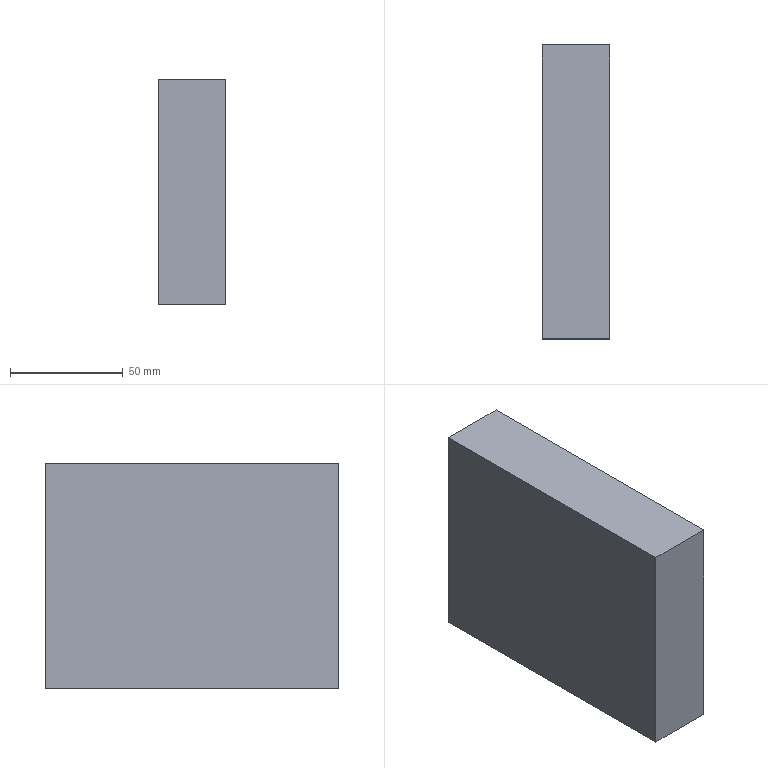Part | Creo | 1 solid | 6 faces | box 30 x 130 x 100 mm | volume 390000 mm3 | plane 6
STEP:
#1=CARTESIAN_POINT('',(0.,0.,0.));
#2=DIRECTION('',(0.,0.,1.));
#3=DIRECTION('',(1.,0.,0.));
#4=AXIS2_PLACEMENT_3D('',#1,#2,#3);
#5=CARTESIAN_POINT('',(-683.899,58.794,-131.793));
#6=VERTEX_POINT('',#5);
#7=CARTESIAN_POINT('',(-653.899,58.794,-131.793));
#8=VERTEX_POINT('',#7);
#9=CARTESIAN_POINT('',(-683.899,58.794,-131.793));
#10=DIRECTION('',(1.,0.,0.));
#11=VECTOR('',#10,30.);
#12=LINE('',#9,#11);
#13=EDGE_CURVE('',#6,#8,#12,.T.);
#14=ORIENTED_EDGE('',*,*,#13,.T.);
#15=CARTESIAN_POINT('',(-653.899,58.794,-31.793));
#16=VERTEX_POINT('',#15);
#17=CARTESIAN_POINT('',(-653.899,58.794,-31.793));
#18=DIRECTION('',(0.,0.,-1.));
#19=VECTOR('',#18,100.);
#20=LINE('',#17,#19);
#21=EDGE_CURVE('',#16,#8,#20,.T.);
#22=ORIENTED_EDGE('',*,*,#21,.F.);
#23=CARTESIAN_POINT('',(-683.899,58.794,-31.793));
#24=VERTEX_POINT('',#23);
#25=CARTESIAN_POINT('',(-653.899,58.794,-31.793));
#26=DIRECTION('',(-1.,0.,0.));
#27=VECTOR('',#26,30.);
#28=LINE('',#25,#27);
#29=EDGE_CURVE('',#16,#24,#28,.T.);
#30=ORIENTED_EDGE('',*,*,#29,.T.);
#31=CARTESIAN_POINT('',(-683.899,58.794,-31.793));
#32=DIRECTION('',(0.,0.,-1.));
#33=VECTOR('',#32,100.);
#34=LINE('',#31,#33);
#35=EDGE_CURVE('',#24,#6,#34,.T.);
#36=ORIENTED_EDGE('',*,*,#35,.T.);
#37=EDGE_LOOP('',(#14,#22,#30,#36));
#38=FACE_OUTER_BOUND('',#37,.F.);
#39=CARTESIAN_POINT('',(-730.899,58.794,-82.793));
#40=DIRECTION('',(0.,1.,0.));
#41=DIRECTION('',(0.,0.,1.));
#42=AXIS2_PLACEMENT_3D('',#39,#40,#41);
#43=PLANE('',#42);
#44=ADVANCED_FACE('',(#38),#43,.T.);
#45=CARTESIAN_POINT('',(-653.899,-71.206,-131.793));
#46=VERTEX_POINT('',#45);
#47=CARTESIAN_POINT('',(-653.899,-71.206,-131.793));
#48=DIRECTION('',(0.,1.,0.));
#49=VECTOR('',#48,130.);
#50=LINE('',#47,#49);
#51=EDGE_CURVE('',#46,#8,#50,.T.);
#52=ORIENTED_EDGE('',*,*,#51,.T.);
#53=ORIENTED_EDGE('',*,*,#13,.F.);
#54=CARTESIAN_POINT('',(-683.899,-71.206,-131.793));
#55=VERTEX_POINT('',#54);
#56=CARTESIAN_POINT('',(-683.899,-71.206,-131.793));
#57=DIRECTION('',(0.,1.,0.));
#58=VECTOR('',#57,130.);
#59=LINE('',#56,#58);
#60=EDGE_CURVE('',#55,#6,#59,.T.);
#61=ORIENTED_EDGE('',*,*,#60,.F.);
#62=CARTESIAN_POINT('',(-683.899,-71.206,-131.793));
#63=DIRECTION('',(1.,0.,0.));
#64=VECTOR('',#63,30.);
#65=LINE('',#62,#64);
#66=EDGE_CURVE('',#55,#46,#65,.T.);
#67=ORIENTED_EDGE('',*,*,#66,.T.);
#68=EDGE_LOOP('',(#52,#53,#61,#67));
#69=FACE_OUTER_BOUND('',#68,.F.);
#70=CARTESIAN_POINT('',(-653.899,68.735,-131.793));
#71=DIRECTION('',(0.,0.,1.));
#72=DIRECTION('',(1.,0.,0.));
#73=AXIS2_PLACEMENT_3D('',#70,#71,#72);
#74=PLANE('',#73);
#75=ADVANCED_FACE('',(#69),#74,.F.);
#76=CARTESIAN_POINT('',(-653.899,-71.206,-31.793));
#77=VERTEX_POINT('',#76);
#78=CARTESIAN_POINT('',(-653.899,-71.206,-31.793));
#79=DIRECTION('',(0.,0.,-1.));
#80=VECTOR('',#79,100.);
#81=LINE('',#78,#80);
#82=EDGE_CURVE('',#77,#46,#81,.T.);
#83=ORIENTED_EDGE('',*,*,#82,.F.);
#84=CARTESIAN_POINT('',(-653.899,-71.206,-31.793));
#85=DIRECTION('',(0.,1.,0.));
#86=VECTOR('',#85,130.);
#87=LINE('',#84,#86);
#88=EDGE_CURVE('',#77,#16,#87,.T.);
#89=ORIENTED_EDGE('',*,*,#88,.T.);
#90=ORIENTED_EDGE('',*,*,#21,.T.);
#91=ORIENTED_EDGE('',*,*,#51,.F.);
#92=EDGE_LOOP('',(#83,#89,#90,#91));
#93=FACE_OUTER_BOUND('',#92,.F.);
#94=CARTESIAN_POINT('',(-653.899,68.735,223.207));
#95=DIRECTION('',(1.,0.,0.));
#96=DIRECTION('',(0.,0.,-1.));
#97=AXIS2_PLACEMENT_3D('',#94,#95,#96);
#98=PLANE('',#97);
#99=ADVANCED_FACE('',(#93),#98,.T.);
#100=ORIENTED_EDGE('',*,*,#82,.T.);
#101=ORIENTED_EDGE('',*,*,#66,.F.);
#102=CARTESIAN_POINT('',(-683.899,-71.206,-31.793));
#103=VERTEX_POINT('',#102);
#104=CARTESIAN_POINT('',(-683.899,-71.206,-31.793));
#105=DIRECTION('',(0.,0.,-1.));
#106=VECTOR('',#105,100.);
#107=LINE('',#104,#106);
#108=EDGE_CURVE('',#103,#55,#107,.T.);
#109=ORIENTED_EDGE('',*,*,#108,.F.);
#110=CARTESIAN_POINT('',(-653.899,-71.206,-31.793));
#111=DIRECTION('',(-1.,0.,0.));
#112=VECTOR('',#111,30.);
#113=LINE('',#110,#112);
#114=EDGE_CURVE('',#77,#103,#113,.T.);
#115=ORIENTED_EDGE('',*,*,#114,.F.);
#116=EDGE_LOOP('',(#100,#101,#109,#115));
#117=FACE_OUTER_BOUND('',#116,.F.);
#118=CARTESIAN_POINT('',(-730.899,-71.206,-82.793));
#119=DIRECTION('',(0.,1.,0.));
#120=DIRECTION('',(0.,0.,1.));
#121=AXIS2_PLACEMENT_3D('',#118,#119,#120);
#122=PLANE('',#121);
#123=ADVANCED_FACE('',(#117),#122,.F.);
#124=ORIENTED_EDGE('',*,*,#60,.T.);
#125=ORIENTED_EDGE('',*,*,#35,.F.);
#126=CARTESIAN_POINT('',(-683.899,-71.206,-31.793));
#127=DIRECTION('',(0.,1.,0.));
#128=VECTOR('',#127,130.);
#129=LINE('',#126,#128);
#130=EDGE_CURVE('',#103,#24,#129,.T.);
#131=ORIENTED_EDGE('',*,*,#130,.F.);
#132=ORIENTED_EDGE('',*,*,#108,.T.);
#133=EDGE_LOOP('',(#124,#125,#131,#132));
#134=FACE_OUTER_BOUND('',#133,.F.);
#135=CARTESIAN_POINT('',(-683.899,68.735,223.207));
#136=DIRECTION('',(1.,0.,0.));
#137=DIRECTION('',(0.,0.,-1.));
#138=AXIS2_PLACEMENT_3D('',#135,#136,#137);
#139=PLANE('',#138);
#140=ADVANCED_FACE('',(#134),#139,.F.);
#141=ORIENTED_EDGE('',*,*,#130,.T.);
#142=ORIENTED_EDGE('',*,*,#29,.F.);
#143=ORIENTED_EDGE('',*,*,#88,.F.);
#144=ORIENTED_EDGE('',*,*,#114,.T.);
#145=EDGE_LOOP('',(#141,#142,#143,#144));
#146=FACE_OUTER_BOUND('',#145,.F.);
#147=CARTESIAN_POINT('',(-653.899,68.735,-31.793));
#148=DIRECTION('',(0.,0.,1.));
#149=DIRECTION('',(1.,0.,0.));
#150=AXIS2_PLACEMENT_3D('',#147,#148,#149);
#151=PLANE('',#150);
#152=ADVANCED_FACE('',(#146),#151,.T.);
#153=CLOSED_SHELL('',(#44,#75,#99,#123,#140,#152));
#154=MANIFOLD_SOLID_BREP('',#153);
#155=(LENGTH_UNIT()NAMED_UNIT(*)SI_UNIT(.MILLI.,.METRE.));
#156=UNCERTAINTY_MEASURE_WITH_UNIT(LENGTH_MEASURE(0.01667),#155,'','');
#157=(NAMED_UNIT(*)PLANE_ANGLE_UNIT()SI_UNIT($,.RADIAN.));
#158=PLANE_ANGLE_MEASURE_WITH_UNIT(PLANE_ANGLE_MEASURE(0.01745),#157);
#159=(CONVERSION_BASED_UNIT('DEGREE',#158)NAMED_UNIT(*)PLANE_ANGLE_UNIT());
#160=(NAMED_UNIT(*)SI_UNIT($,.STERADIAN.)SOLID_ANGLE_UNIT());
#161=(GEOMETRIC_REPRESENTATION_CONTEXT(3)GLOBAL_UNCERTAINTY_ASSIGNED_CONTEXT((#156))GLOBAL_UNIT_ASSIGNED_CONTEXT((#155,#159,#160))REPRESENTATION_CONTEXT('',''));
#162=ADVANCED_BREP_SHAPE_REPRESENTATION('',(#4,#154),#161);